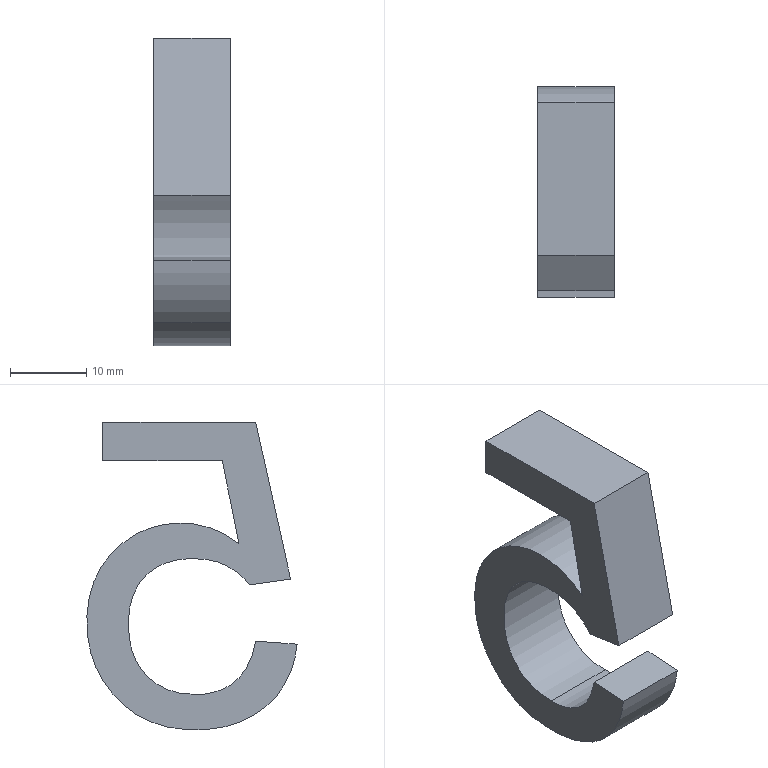Part | NX | features solid 2 | 1 solid | 14 faces | box 10 x 27.61 x 40.382 mm | volume 4846 mm3 | plane 9 | spline 5
STEP:
#1=CARTESIAN_POINT('',(2250.,-233.508,-587.73));
#2=VERTEX_POINT('',#1);
#3=CARTESIAN_POINT('',(2250.,-237.6,-579.522));
#4=VERTEX_POINT('',#3);
#5=CARTESIAN_POINT('',(2250.,-233.508,-587.73));
#6=CARTESIAN_POINT('',(2250.,-235.902,-585.686));
#7=CARTESIAN_POINT('',(2250.,-237.263,-582.948));
#8=CARTESIAN_POINT('',(2250.,-237.6,-579.522));
#9=B_SPLINE_CURVE_WITH_KNOTS('',3,(#5,#6,#7,#8),.UNSPECIFIED.,.F.,.F.,(4,4),(0.,0.04563),.PIECEWISE_BEZIER_KNOTS.);
#10=EDGE_CURVE('',#2,#4,#9,.T.);
#11=ORIENTED_EDGE('',*,*,#10,.F.);
#12=CARTESIAN_POINT('',(2260.,-233.508,-587.73));
#13=VERTEX_POINT('',#12);
#14=CARTESIAN_POINT('',(2260.,-233.508,-587.73));
#15=DIRECTION('',(-1.,0.,0.));
#16=VECTOR('',#15,1000.);
#17=LINE('',#14,#16);
#18=EDGE_CURVE('',#13,#2,#17,.T.);
#19=ORIENTED_EDGE('',*,*,#18,.F.);
#20=CARTESIAN_POINT('',(2260.,-237.6,-579.522));
#21=VERTEX_POINT('',#20);
#22=CARTESIAN_POINT('',(2260.,-233.508,-587.73));
#23=CARTESIAN_POINT('',(2260.,-235.902,-585.686));
#24=CARTESIAN_POINT('',(2260.,-237.263,-582.948));
#25=CARTESIAN_POINT('',(2260.,-237.6,-579.522));
#26=B_SPLINE_CURVE_WITH_KNOTS('',3,(#22,#23,#24,#25),.UNSPECIFIED.,.F.,.F.,(4,4),(0.,0.04563),.PIECEWISE_BEZIER_KNOTS.);
#27=EDGE_CURVE('',#13,#21,#26,.T.);
#28=ORIENTED_EDGE('',*,*,#27,.T.);
#29=CARTESIAN_POINT('',(2260.,-237.6,-579.522));
#30=DIRECTION('',(-1.,0.,0.));
#31=VECTOR('',#30,1000.);
#32=LINE('',#29,#31);
#33=EDGE_CURVE('',#21,#4,#32,.T.);
#34=ORIENTED_EDGE('',*,*,#33,.T.);
#35=EDGE_LOOP('',(#11,#19,#28,#34));
#36=FACE_BOUND('',#35,.T.);
#37=CARTESIAN_POINT('',(2260.,-233.508,-587.73));
#38=CARTESIAN_POINT('',(2250.,-233.508,-587.73));
#39=CARTESIAN_POINT('',(2260.,-235.902,-585.686));
#40=CARTESIAN_POINT('',(2250.,-235.902,-585.686));
#41=CARTESIAN_POINT('',(2260.,-237.263,-582.948));
#42=CARTESIAN_POINT('',(2250.,-237.263,-582.948));
#43=CARTESIAN_POINT('',(2260.,-237.6,-579.522));
#44=CARTESIAN_POINT('',(2250.,-237.6,-579.522));
#45=B_SPLINE_SURFACE_WITH_KNOTS('',3,1,((#37,#38),(#39,#40),(#41,#42),(#43,#44)),.SURF_OF_LINEAR_EXTRUSION.,.F.,.F.,.F.,(4,4),(2,2),(0.,0.04563),(0.,1.),.PIECEWISE_BEZIER_KNOTS.);
#46=ADVANCED_FACE('',(#36),#45,.T.);
#47=CARTESIAN_POINT('',(2250.,-232.17,-579.124));
#48=VERTEX_POINT('',#47);
#49=CARTESIAN_POINT('',(2250.,-237.6,-579.522));
#50=CARTESIAN_POINT('',(2250.,-235.79,-579.389));
#51=CARTESIAN_POINT('',(2250.,-233.98,-579.257));
#52=CARTESIAN_POINT('',(2250.,-232.17,-579.124));
#53=B_SPLINE_CURVE_WITH_KNOTS('',3,(#49,#50,#51,#52),.UNSPECIFIED.,.F.,.F.,(4,4),(0.04563,0.07202),.PIECEWISE_BEZIER_KNOTS.);
#54=EDGE_CURVE('',#4,#48,#53,.T.);
#55=ORIENTED_EDGE('',*,*,#54,.F.);
#56=ORIENTED_EDGE('',*,*,#33,.F.);
#57=CARTESIAN_POINT('',(2260.,-232.17,-579.124));
#58=VERTEX_POINT('',#57);
#59=CARTESIAN_POINT('',(2260.,-237.6,-579.522));
#60=CARTESIAN_POINT('',(2260.,-235.79,-579.389));
#61=CARTESIAN_POINT('',(2260.,-233.98,-579.257));
#62=CARTESIAN_POINT('',(2260.,-232.17,-579.124));
#63=B_SPLINE_CURVE_WITH_KNOTS('',3,(#59,#60,#61,#62),.UNSPECIFIED.,.F.,.F.,(4,4),(0.04563,0.07202),.PIECEWISE_BEZIER_KNOTS.);
#64=EDGE_CURVE('',#21,#58,#63,.T.);
#65=ORIENTED_EDGE('',*,*,#64,.T.);
#66=CARTESIAN_POINT('',(2260.,-232.17,-579.124));
#67=DIRECTION('',(-1.,0.,0.));
#68=VECTOR('',#67,1000.);
#69=LINE('',#66,#68);
#70=EDGE_CURVE('',#58,#48,#69,.T.);
#71=ORIENTED_EDGE('',*,*,#70,.T.);
#72=EDGE_LOOP('',(#55,#56,#65,#71));
#73=FACE_BOUND('',#72,.T.);
#74=CARTESIAN_POINT('',(2260.,-237.6,-579.522));
#75=DIRECTION('',(0.,-0.07304,0.9973));
#76=DIRECTION('',(0.,-0.9973,-0.07304));
#77=AXIS2_PLACEMENT_3D('',#74,#75,#76);
#78=PLANE('',#77);
#79=ADVANCED_FACE('',(#73),#78,.T.);
#80=CARTESIAN_POINT('',(2250.,-224.216,-586.115));
#81=VERTEX_POINT('',#80);
#82=CARTESIAN_POINT('',(2250.,-232.17,-579.124));
#83=CARTESIAN_POINT('',(2250.,-231.772,-581.48));
#84=CARTESIAN_POINT('',(2250.,-230.885,-583.239));
#85=CARTESIAN_POINT('',(2250.,-228.153,-585.572));
#86=CARTESIAN_POINT('',(2250.,-226.357,-586.145));
#87=CARTESIAN_POINT('',(2250.,-224.216,-586.115));
#88=B_SPLINE_CURVE_WITH_KNOTS('',3,(#82,#83,#84,#85,#86,#87),.UNSPECIFIED.,.F.,.F.,(4,2,4),(0.07202,0.1012,0.1307),.UNSPECIFIED.);
#89=EDGE_CURVE('',#48,#81,#88,.T.);
#90=ORIENTED_EDGE('',*,*,#89,.F.);
#91=ORIENTED_EDGE('',*,*,#70,.F.);
#92=CARTESIAN_POINT('',(2260.,-224.216,-586.115));
#93=VERTEX_POINT('',#92);
#94=CARTESIAN_POINT('',(2260.,-232.17,-579.124));
#95=CARTESIAN_POINT('',(2260.,-231.772,-581.48));
#96=CARTESIAN_POINT('',(2260.,-230.885,-583.239));
#97=CARTESIAN_POINT('',(2260.,-228.153,-585.572));
#98=CARTESIAN_POINT('',(2260.,-226.357,-586.145));
#99=CARTESIAN_POINT('',(2260.,-224.216,-586.115));
#100=B_SPLINE_CURVE_WITH_KNOTS('',3,(#94,#95,#96,#97,#98,#99),.UNSPECIFIED.,.F.,.F.,(4,2,4),(0.07202,0.1012,0.1307),.UNSPECIFIED.);
#101=EDGE_CURVE('',#58,#93,#100,.T.);
#102=ORIENTED_EDGE('',*,*,#101,.T.);
#103=CARTESIAN_POINT('',(2260.,-224.216,-586.115));
#104=DIRECTION('',(-1.,0.,0.));
#105=VECTOR('',#104,1000.);
#106=LINE('',#103,#105);
#107=EDGE_CURVE('',#93,#81,#106,.T.);
#108=ORIENTED_EDGE('',*,*,#107,.T.);
#109=EDGE_LOOP('',(#90,#91,#102,#108));
#110=FACE_BOUND('',#109,.T.);
#111=CARTESIAN_POINT('',(2260.,-232.17,-579.124));
#112=CARTESIAN_POINT('',(2250.,-232.17,-579.124));
#113=CARTESIAN_POINT('',(2260.,-231.372,-583.851));
#114=CARTESIAN_POINT('',(2250.,-231.372,-583.851));
#115=CARTESIAN_POINT('',(2260.,-228.485,-586.176));
#116=CARTESIAN_POINT('',(2250.,-228.485,-586.176));
#117=CARTESIAN_POINT('',(2260.,-224.216,-586.115));
#118=CARTESIAN_POINT('',(2250.,-224.216,-586.115));
#119=B_SPLINE_SURFACE_WITH_KNOTS('',3,1,((#111,#112),(#113,#114),(#115,#116),(#117,#118)),.SURF_OF_LINEAR_EXTRUSION.,.F.,.F.,.F.,(4,4),(2,2),(0.07202,0.1307),(0.,1.),.PIECEWISE_BEZIER_KNOTS.);
#120=ADVANCED_FACE('',(#110),#119,.T.);
#121=CARTESIAN_POINT('',(2250.,-231.328,-571.751));
#122=VERTEX_POINT('',#121);
#123=CARTESIAN_POINT('',(2250.,-224.216,-586.115));
#124=CARTESIAN_POINT('',(2250.,-221.554,-586.145));
#125=CARTESIAN_POINT('',(2250.,-219.413,-585.304));
#126=CARTESIAN_POINT('',(2250.,-217.799,-583.598));
#127=CARTESIAN_POINT('',(2250.,-216.216,-581.924));
#128=CARTESIAN_POINT('',(2250.,-215.436,-579.69));
#129=CARTESIAN_POINT('',(2250.,-215.436,-574.229));
#130=CARTESIAN_POINT('',(2250.,-216.17,-572.134));
#131=CARTESIAN_POINT('',(2250.,-219.122,-569.06));
#132=CARTESIAN_POINT('',(2250.,-221.233,-568.279));
#133=CARTESIAN_POINT('',(2250.,-224.002,-568.279));
#134=CARTESIAN_POINT('',(2250.,-225.73,-568.279));
#135=CARTESIAN_POINT('',(2250.,-227.229,-568.616));
#136=CARTESIAN_POINT('',(2250.,-229.627,-569.907));
#137=CARTESIAN_POINT('',(2250.,-230.594,-570.727));
#138=CARTESIAN_POINT('',(2250.,-231.328,-571.751));
#139=B_SPLINE_CURVE_WITH_KNOTS('',3,(#123,#124,#125,#126,#127,#128,#129,#130,#131,#132,#133,#134,#135,#136,#137,#138),.UNSPECIFIED.,.F.,.F.,(4,3,2,2,3,2,4),(0.1307,0.1656,0.2015,0.2352,0.2686,0.2911,0.3137),.UNSPECIFIED.);
#140=EDGE_CURVE('',#81,#122,#139,.T.);
#141=ORIENTED_EDGE('',*,*,#140,.F.);
#142=ORIENTED_EDGE('',*,*,#107,.F.);
#143=CARTESIAN_POINT('',(2260.,-231.328,-571.751));
#144=VERTEX_POINT('',#143);
#145=CARTESIAN_POINT('',(2260.,-224.216,-586.115));
#146=CARTESIAN_POINT('',(2260.,-221.554,-586.145));
#147=CARTESIAN_POINT('',(2260.,-219.413,-585.304));
#148=CARTESIAN_POINT('',(2260.,-217.799,-583.598));
#149=CARTESIAN_POINT('',(2260.,-216.216,-581.924));
#150=CARTESIAN_POINT('',(2260.,-215.436,-579.69));
#151=CARTESIAN_POINT('',(2260.,-215.436,-574.229));
#152=CARTESIAN_POINT('',(2260.,-216.17,-572.134));
#153=CARTESIAN_POINT('',(2260.,-219.122,-569.06));
#154=CARTESIAN_POINT('',(2260.,-221.233,-568.279));
#155=CARTESIAN_POINT('',(2260.,-224.002,-568.279));
#156=CARTESIAN_POINT('',(2260.,-225.73,-568.279));
#157=CARTESIAN_POINT('',(2260.,-227.229,-568.616));
#158=CARTESIAN_POINT('',(2260.,-229.627,-569.907));
#159=CARTESIAN_POINT('',(2260.,-230.594,-570.727));
#160=CARTESIAN_POINT('',(2260.,-231.328,-571.751));
#161=B_SPLINE_CURVE_WITH_KNOTS('',3,(#145,#146,#147,#148,#149,#150,#151,#152,#153,#154,#155,#156,#157,#158,#159,#160),.UNSPECIFIED.,.F.,.F.,(4,3,2,2,3,2,4),(0.1307,0.1656,0.2015,0.2352,0.2686,0.2911,0.3137),.UNSPECIFIED.);
#162=EDGE_CURVE('',#93,#144,#161,.T.);
#163=ORIENTED_EDGE('',*,*,#162,.T.);
#164=CARTESIAN_POINT('',(2260.,-231.328,-571.751));
#165=DIRECTION('',(-1.,0.,0.));
#166=VECTOR('',#165,1000.);
#167=LINE('',#164,#166);
#168=EDGE_CURVE('',#144,#122,#167,.T.);
#169=ORIENTED_EDGE('',*,*,#168,.T.);
#170=EDGE_LOOP('',(#141,#142,#163,#169));
#171=FACE_BOUND('',#170,.T.);
#172=CARTESIAN_POINT('',(2260.,-224.216,-586.115));
#173=CARTESIAN_POINT('',(2250.,-224.216,-586.115));
#174=CARTESIAN_POINT('',(2260.,-222.471,-586.135));
#175=CARTESIAN_POINT('',(2250.,-222.471,-586.135));
#176=CARTESIAN_POINT('',(2260.,-220.207,-585.624));
#177=CARTESIAN_POINT('',(2250.,-220.207,-585.624));
#178=CARTESIAN_POINT('',(2260.,-217.794,-583.741));
#179=CARTESIAN_POINT('',(2250.,-217.794,-583.741));
#180=CARTESIAN_POINT('',(2260.,-216.501,-581.979));
#181=CARTESIAN_POINT('',(2250.,-216.501,-581.979));
#182=CARTESIAN_POINT('',(2260.,-215.693,-579.891));
#183=CARTESIAN_POINT('',(2250.,-215.693,-579.891));
#184=CARTESIAN_POINT('',(2260.,-215.364,-577.41));
#185=CARTESIAN_POINT('',(2250.,-215.364,-577.41));
#186=CARTESIAN_POINT('',(2260.,-215.517,-574.731));
#187=CARTESIAN_POINT('',(2250.,-215.517,-574.731));
#188=CARTESIAN_POINT('',(2260.,-216.183,-572.568));
#189=CARTESIAN_POINT('',(2250.,-216.183,-572.568));
#190=CARTESIAN_POINT('',(2260.,-217.367,-570.739));
#191=CARTESIAN_POINT('',(2250.,-217.367,-570.739));
#192=CARTESIAN_POINT('',(2260.,-219.045,-569.339));
#193=CARTESIAN_POINT('',(2250.,-219.045,-569.339));
#194=CARTESIAN_POINT('',(2260.,-220.823,-568.637));
#195=CARTESIAN_POINT('',(2250.,-220.823,-568.637));
#196=CARTESIAN_POINT('',(2260.,-222.455,-568.342));
#197=CARTESIAN_POINT('',(2250.,-222.455,-568.342));
#198=CARTESIAN_POINT('',(2260.,-224.316,-568.23));
#199=CARTESIAN_POINT('',(2250.,-224.316,-568.23));
#200=CARTESIAN_POINT('',(2260.,-226.396,-568.42));
#201=CARTESIAN_POINT('',(2250.,-226.396,-568.42));
#202=CARTESIAN_POINT('',(2260.,-228.457,-569.176));
#203=CARTESIAN_POINT('',(2250.,-228.457,-569.176));
#204=CARTESIAN_POINT('',(2260.,-230.095,-570.309));
#205=CARTESIAN_POINT('',(2250.,-230.095,-570.309));
#206=CARTESIAN_POINT('',(2260.,-230.958,-571.234));
#207=CARTESIAN_POINT('',(2250.,-230.958,-571.234));
#208=CARTESIAN_POINT('',(2260.,-231.328,-571.751));
#209=CARTESIAN_POINT('',(2250.,-231.328,-571.751));
#210=B_SPLINE_SURFACE_WITH_KNOTS('',3,1,((#172,#173),(#174,#175),(#176,#177),(#178,#179),(#180,#181),(#182,#183),(#184,#185),(#186,#187),(#188,#189),(#190,#191),(#192,#193),(#194,#195),(#196,#197),(#198,#199),(#200,#201),(#202,#203),(#204,#205),(#206,#207),(#208,#209)),.SURF_OF_LINEAR_EXTRUSION.,.F.,.F.,.F.,(4,1,1,1,1,1,1,1,1,1,1,1,1,1,1,1,4),(2,2),(0.1307,0.1535,0.165,0.1764,0.1879,0.1993,0.2107,0.2222,0.2336,0.2451,0.2565,0.2622,0.268,0.2794,0.2908,0.3023,0.3137),(0.,1.),.UNSPECIFIED.);
#211=ADVANCED_FACE('',(#171),#210,.T.);
#212=CARTESIAN_POINT('',(2250.,-236.759,-570.971));
#213=VERTEX_POINT('',#212);
#214=CARTESIAN_POINT('',(2250.,-231.328,-571.751));
#215=CARTESIAN_POINT('',(2250.,-233.139,-571.491));
#216=CARTESIAN_POINT('',(2250.,-234.949,-571.231));
#217=CARTESIAN_POINT('',(2250.,-236.759,-570.971));
#218=B_SPLINE_CURVE_WITH_KNOTS('',3,(#214,#215,#216,#217),.UNSPECIFIED.,.F.,.F.,(4,4),(0.3137,0.341),.PIECEWISE_BEZIER_KNOTS.);
#219=EDGE_CURVE('',#122,#213,#218,.T.);
#220=ORIENTED_EDGE('',*,*,#219,.F.);
#221=ORIENTED_EDGE('',*,*,#168,.F.);
#222=CARTESIAN_POINT('',(2260.,-236.759,-570.971));
#223=VERTEX_POINT('',#222);
#224=CARTESIAN_POINT('',(2260.,-231.328,-571.751));
#225=CARTESIAN_POINT('',(2260.,-233.139,-571.491));
#226=CARTESIAN_POINT('',(2260.,-234.949,-571.231));
#227=CARTESIAN_POINT('',(2260.,-236.759,-570.971));
#228=B_SPLINE_CURVE_WITH_KNOTS('',3,(#224,#225,#226,#227),.UNSPECIFIED.,.F.,.F.,(4,4),(0.3137,0.341),.PIECEWISE_BEZIER_KNOTS.);
#229=EDGE_CURVE('',#144,#223,#228,.T.);
#230=ORIENTED_EDGE('',*,*,#229,.T.);
#231=CARTESIAN_POINT('',(2260.,-236.759,-570.971));
#232=DIRECTION('',(-1.,0.,0.));
#233=VECTOR('',#232,1000.);
#234=LINE('',#231,#233);
#235=EDGE_CURVE('',#223,#213,#234,.T.);
#236=ORIENTED_EDGE('',*,*,#235,.T.);
#237=EDGE_LOOP('',(#220,#221,#230,#236));
#238=FACE_BOUND('',#237,.T.);
#239=CARTESIAN_POINT('',(2260.,-231.328,-571.751));
#240=DIRECTION('',(0.,-0.1422,-0.9898));
#241=DIRECTION('',(0.,0.9898,-0.1422));
#242=AXIS2_PLACEMENT_3D('',#239,#240,#241);
#243=PLANE('',#242);
#244=ADVANCED_FACE('',(#238),#243,.T.);
#245=CARTESIAN_POINT('',(2250.,-232.17,-550.398));
#246=VERTEX_POINT('',#245);
#247=CARTESIAN_POINT('',(2250.,-236.759,-570.971));
#248=CARTESIAN_POINT('',(2250.,-235.229,-564.113));
#249=CARTESIAN_POINT('',(2250.,-233.699,-557.256));
#250=CARTESIAN_POINT('',(2250.,-232.17,-550.398));
#251=B_SPLINE_CURVE_WITH_KNOTS('',3,(#247,#248,#249,#250),.UNSPECIFIED.,.F.,.F.,(4,4),(0.341,0.4456),.PIECEWISE_BEZIER_KNOTS.);
#252=EDGE_CURVE('',#213,#246,#251,.T.);
#253=ORIENTED_EDGE('',*,*,#252,.F.);
#254=ORIENTED_EDGE('',*,*,#235,.F.);
#255=CARTESIAN_POINT('',(2260.,-232.17,-550.398));
#256=VERTEX_POINT('',#255);
#257=CARTESIAN_POINT('',(2260.,-236.759,-570.971));
#258=CARTESIAN_POINT('',(2260.,-235.229,-564.113));
#259=CARTESIAN_POINT('',(2260.,-233.699,-557.256));
#260=CARTESIAN_POINT('',(2260.,-232.17,-550.398));
#261=B_SPLINE_CURVE_WITH_KNOTS('',3,(#257,#258,#259,#260),.UNSPECIFIED.,.F.,.F.,(4,4),(0.341,0.4456),.PIECEWISE_BEZIER_KNOTS.);
#262=EDGE_CURVE('',#223,#256,#261,.T.);
#263=ORIENTED_EDGE('',*,*,#262,.T.);
#264=CARTESIAN_POINT('',(2260.,-232.17,-550.398));
#265=DIRECTION('',(-1.,0.,0.));
#266=VECTOR('',#265,1000.);
#267=LINE('',#264,#266);
#268=EDGE_CURVE('',#256,#246,#267,.T.);
#269=ORIENTED_EDGE('',*,*,#268,.T.);
#270=EDGE_LOOP('',(#253,#254,#263,#269));
#271=FACE_BOUND('',#270,.T.);
#272=CARTESIAN_POINT('',(2260.,-236.759,-570.971));
#273=DIRECTION('',(0.,-0.976,0.2177));
#274=DIRECTION('',(0.,-0.2177,-0.976));
#275=AXIS2_PLACEMENT_3D('',#272,#273,#274);
#276=PLANE('',#275);
#277=ADVANCED_FACE('',(#271),#276,.T.);
#278=CARTESIAN_POINT('',(2250.,-212.086,-550.398));
#279=VERTEX_POINT('',#278);
#280=CARTESIAN_POINT('',(2250.,-232.17,-550.398));
#281=CARTESIAN_POINT('',(2250.,-225.475,-550.398));
#282=CARTESIAN_POINT('',(2250.,-218.78,-550.398));
#283=CARTESIAN_POINT('',(2250.,-212.086,-550.398));
#284=B_SPLINE_CURVE_WITH_KNOTS('',3,(#280,#281,#282,#283),.UNSPECIFIED.,.F.,.F.,(4,4),(0.4456,0.5452),.PIECEWISE_BEZIER_KNOTS.);
#285=EDGE_CURVE('',#246,#279,#284,.T.);
#286=ORIENTED_EDGE('',*,*,#285,.F.);
#287=ORIENTED_EDGE('',*,*,#268,.F.);
#288=CARTESIAN_POINT('',(2260.,-212.086,-550.398));
#289=VERTEX_POINT('',#288);
#290=CARTESIAN_POINT('',(2260.,-232.17,-550.398));
#291=CARTESIAN_POINT('',(2260.,-225.475,-550.398));
#292=CARTESIAN_POINT('',(2260.,-218.78,-550.398));
#293=CARTESIAN_POINT('',(2260.,-212.086,-550.398));
#294=B_SPLINE_CURVE_WITH_KNOTS('',3,(#290,#291,#292,#293),.UNSPECIFIED.,.F.,.F.,(4,4),(0.4456,0.5452),.PIECEWISE_BEZIER_KNOTS.);
#295=EDGE_CURVE('',#256,#289,#294,.T.);
#296=ORIENTED_EDGE('',*,*,#295,.T.);
#297=CARTESIAN_POINT('',(2260.,-212.086,-550.398));
#298=DIRECTION('',(-1.,0.,0.));
#299=VECTOR('',#298,1000.);
#300=LINE('',#297,#299);
#301=EDGE_CURVE('',#289,#279,#300,.T.);
#302=ORIENTED_EDGE('',*,*,#301,.T.);
#303=EDGE_LOOP('',(#286,#287,#296,#302));
#304=FACE_BOUND('',#303,.T.);
#305=CARTESIAN_POINT('',(2260.,-232.17,-550.398));
#306=DIRECTION('',(0.,0.,1.));
#307=DIRECTION('',(1.,0.,0.));
#308=AXIS2_PLACEMENT_3D('',#305,#306,#307);
#309=PLANE('',#308);
#310=ADVANCED_FACE('',(#304),#309,.T.);
#311=CARTESIAN_POINT('',(2250.,-212.086,-555.446));
#312=VERTEX_POINT('',#311);
#313=CARTESIAN_POINT('',(2250.,-212.086,-550.398));
#314=CARTESIAN_POINT('',(2250.,-212.086,-552.08));
#315=CARTESIAN_POINT('',(2250.,-212.086,-553.763));
#316=CARTESIAN_POINT('',(2250.,-212.086,-555.446));
#317=B_SPLINE_CURVE_WITH_KNOTS('',3,(#313,#314,#315,#316),.UNSPECIFIED.,.F.,.F.,(4,4),(0.5452,0.5703),.PIECEWISE_BEZIER_KNOTS.);
#318=EDGE_CURVE('',#279,#312,#317,.T.);
#319=ORIENTED_EDGE('',*,*,#318,.F.);
#320=ORIENTED_EDGE('',*,*,#301,.F.);
#321=CARTESIAN_POINT('',(2260.,-212.086,-555.446));
#322=VERTEX_POINT('',#321);
#323=CARTESIAN_POINT('',(2260.,-212.086,-550.398));
#324=CARTESIAN_POINT('',(2260.,-212.086,-552.08));
#325=CARTESIAN_POINT('',(2260.,-212.086,-553.763));
#326=CARTESIAN_POINT('',(2260.,-212.086,-555.446));
#327=B_SPLINE_CURVE_WITH_KNOTS('',3,(#323,#324,#325,#326),.UNSPECIFIED.,.F.,.F.,(4,4),(0.5452,0.5703),.PIECEWISE_BEZIER_KNOTS.);
#328=EDGE_CURVE('',#289,#322,#327,.T.);
#329=ORIENTED_EDGE('',*,*,#328,.T.);
#330=CARTESIAN_POINT('',(2260.,-212.086,-555.446));
#331=DIRECTION('',(-1.,0.,0.));
#332=VECTOR('',#331,1000.);
#333=LINE('',#330,#332);
#334=EDGE_CURVE('',#322,#312,#333,.T.);
#335=ORIENTED_EDGE('',*,*,#334,.T.);
#336=EDGE_LOOP('',(#319,#320,#329,#335));
#337=FACE_BOUND('',#336,.T.);
#338=CARTESIAN_POINT('',(2260.,-212.086,-550.398));
#339=DIRECTION('',(0.,1.,0.));
#340=DIRECTION('',(-1.,0.,0.));
#341=AXIS2_PLACEMENT_3D('',#338,#339,#340);
#342=PLANE('',#341);
#343=ADVANCED_FACE('',(#337),#342,.T.);
#344=CARTESIAN_POINT('',(2250.,-227.78,-555.446));
#345=VERTEX_POINT('',#344);
#346=CARTESIAN_POINT('',(2250.,-212.086,-555.446));
#347=CARTESIAN_POINT('',(2250.,-217.317,-555.446));
#348=CARTESIAN_POINT('',(2250.,-222.548,-555.446));
#349=CARTESIAN_POINT('',(2250.,-227.78,-555.446));
#350=B_SPLINE_CURVE_WITH_KNOTS('',3,(#346,#347,#348,#349),.UNSPECIFIED.,.F.,.F.,(4,4),(0.5703,0.6481),.PIECEWISE_BEZIER_KNOTS.);
#351=EDGE_CURVE('',#312,#345,#350,.T.);
#352=ORIENTED_EDGE('',*,*,#351,.F.);
#353=ORIENTED_EDGE('',*,*,#334,.F.);
#354=CARTESIAN_POINT('',(2260.,-227.78,-555.446));
#355=VERTEX_POINT('',#354);
#356=CARTESIAN_POINT('',(2260.,-212.086,-555.446));
#357=CARTESIAN_POINT('',(2260.,-217.317,-555.446));
#358=CARTESIAN_POINT('',(2260.,-222.548,-555.446));
#359=CARTESIAN_POINT('',(2260.,-227.78,-555.446));
#360=B_SPLINE_CURVE_WITH_KNOTS('',3,(#356,#357,#358,#359),.UNSPECIFIED.,.F.,.F.,(4,4),(0.5703,0.6481),.PIECEWISE_BEZIER_KNOTS.);
#361=EDGE_CURVE('',#322,#355,#360,.T.);
#362=ORIENTED_EDGE('',*,*,#361,.T.);
#363=CARTESIAN_POINT('',(2260.,-227.78,-555.446));
#364=DIRECTION('',(-1.,0.,0.));
#365=VECTOR('',#364,1000.);
#366=LINE('',#363,#365);
#367=EDGE_CURVE('',#355,#345,#366,.T.);
#368=ORIENTED_EDGE('',*,*,#367,.T.);
#369=EDGE_LOOP('',(#352,#353,#362,#368));
#370=FACE_BOUND('',#369,.T.);
#371=CARTESIAN_POINT('',(2260.,-212.086,-555.446));
#372=DIRECTION('',(0.,0.,-1.));
#373=DIRECTION('',(-1.,0.,0.));
#374=AXIS2_PLACEMENT_3D('',#371,#372,#373);
#375=PLANE('',#374);
#376=ADVANCED_FACE('',(#370),#375,.T.);
#377=CARTESIAN_POINT('',(2250.,-229.967,-566.291));
#378=VERTEX_POINT('',#377);
#379=CARTESIAN_POINT('',(2250.,-227.78,-555.446));
#380=CARTESIAN_POINT('',(2250.,-228.509,-559.061));
#381=CARTESIAN_POINT('',(2250.,-229.238,-562.676));
#382=CARTESIAN_POINT('',(2250.,-229.967,-566.291));
#383=B_SPLINE_CURVE_WITH_KNOTS('',3,(#379,#380,#381,#382),.UNSPECIFIED.,.F.,.F.,(4,4),(0.6481,0.703),.PIECEWISE_BEZIER_KNOTS.);
#384=EDGE_CURVE('',#345,#378,#383,.T.);
#385=ORIENTED_EDGE('',*,*,#384,.F.);
#386=ORIENTED_EDGE('',*,*,#367,.F.);
#387=CARTESIAN_POINT('',(2260.,-229.967,-566.291));
#388=VERTEX_POINT('',#387);
#389=CARTESIAN_POINT('',(2260.,-227.78,-555.446));
#390=CARTESIAN_POINT('',(2260.,-228.509,-559.061));
#391=CARTESIAN_POINT('',(2260.,-229.238,-562.676));
#392=CARTESIAN_POINT('',(2260.,-229.967,-566.291));
#393=B_SPLINE_CURVE_WITH_KNOTS('',3,(#389,#390,#391,#392),.UNSPECIFIED.,.F.,.F.,(4,4),(0.6481,0.703),.PIECEWISE_BEZIER_KNOTS.);
#394=EDGE_CURVE('',#355,#388,#393,.T.);
#395=ORIENTED_EDGE('',*,*,#394,.T.);
#396=CARTESIAN_POINT('',(2260.,-229.967,-566.291));
#397=DIRECTION('',(-1.,0.,0.));
#398=VECTOR('',#397,1000.);
#399=LINE('',#396,#398);
#400=EDGE_CURVE('',#388,#378,#399,.T.);
#401=ORIENTED_EDGE('',*,*,#400,.T.);
#402=EDGE_LOOP('',(#385,#386,#395,#401));
#403=FACE_BOUND('',#402,.T.);
#404=CARTESIAN_POINT('',(2260.,-227.78,-555.446));
#405=DIRECTION('',(0.,0.9803,-0.1977));
#406=DIRECTION('',(0.,0.1977,0.9803));
#407=AXIS2_PLACEMENT_3D('',#404,#405,#406);
#408=PLANE('',#407);
#409=ADVANCED_FACE('',(#403),#408,.T.);
#410=CARTESIAN_POINT('',(2250.,-213.294,-585.931));
#411=VERTEX_POINT('',#410);
#412=CARTESIAN_POINT('',(2250.,-229.967,-566.291));
#413=CARTESIAN_POINT('',(2250.,-227.566,-564.516));
#414=CARTESIAN_POINT('',(2250.,-225.057,-563.614));
#415=CARTESIAN_POINT('',(2250.,-222.441,-563.614));
#416=CARTESIAN_POINT('',(2250.,-218.938,-563.614));
#417=CARTESIAN_POINT('',(2250.,-215.986,-564.837));
#418=CARTESIAN_POINT('',(2250.,-211.16,-569.663));
#419=CARTESIAN_POINT('',(2250.,-209.99,-572.776));
#420=CARTESIAN_POINT('',(2250.,-209.99,-580.195));
#421=CARTESIAN_POINT('',(2250.,-211.091,-583.331));
#422=CARTESIAN_POINT('',(2250.,-213.294,-585.931));
#423=B_SPLINE_CURVE_WITH_KNOTS('',3,(#412,#413,#414,#415,#416,#417,#418,#419,#420,#421,#422),.UNSPECIFIED.,.F.,.F.,(4,3,2,2,4),(0.703,0.7434,0.7922,0.8415,0.889),.UNSPECIFIED.);
#424=EDGE_CURVE('',#378,#411,#423,.T.);
#425=ORIENTED_EDGE('',*,*,#424,.F.);
#426=ORIENTED_EDGE('',*,*,#400,.F.);
#427=CARTESIAN_POINT('',(2260.,-213.294,-585.931));
#428=VERTEX_POINT('',#427);
#429=CARTESIAN_POINT('',(2260.,-229.967,-566.291));
#430=CARTESIAN_POINT('',(2260.,-227.566,-564.516));
#431=CARTESIAN_POINT('',(2260.,-225.057,-563.614));
#432=CARTESIAN_POINT('',(2260.,-222.441,-563.614));
#433=CARTESIAN_POINT('',(2260.,-218.938,-563.614));
#434=CARTESIAN_POINT('',(2260.,-215.986,-564.837));
#435=CARTESIAN_POINT('',(2260.,-211.16,-569.663));
#436=CARTESIAN_POINT('',(2260.,-209.99,-572.776));
#437=CARTESIAN_POINT('',(2260.,-209.99,-580.195));
#438=CARTESIAN_POINT('',(2260.,-211.091,-583.331));
#439=CARTESIAN_POINT('',(2260.,-213.294,-585.931));
#440=B_SPLINE_CURVE_WITH_KNOTS('',3,(#429,#430,#431,#432,#433,#434,#435,#436,#437,#438,#439),.UNSPECIFIED.,.F.,.F.,(4,3,2,2,4),(0.703,0.7434,0.7922,0.8415,0.889),.UNSPECIFIED.);
#441=EDGE_CURVE('',#388,#428,#440,.T.);
#442=ORIENTED_EDGE('',*,*,#441,.T.);
#443=CARTESIAN_POINT('',(2260.,-213.294,-585.931));
#444=DIRECTION('',(-1.,0.,0.));
#445=VECTOR('',#444,1000.);
#446=LINE('',#443,#445);
#447=EDGE_CURVE('',#428,#411,#446,.T.);
#448=ORIENTED_EDGE('',*,*,#447,.T.);
#449=EDGE_LOOP('',(#425,#426,#442,#448));
#450=FACE_BOUND('',#449,.T.);
#451=CARTESIAN_POINT('',(2260.,-229.967,-566.291));
#452=CARTESIAN_POINT('',(2250.,-229.967,-566.291));
#453=CARTESIAN_POINT('',(2260.,-228.584,-565.268));
#454=CARTESIAN_POINT('',(2250.,-228.584,-565.268));
#455=CARTESIAN_POINT('',(2260.,-226.463,-564.17));
#456=CARTESIAN_POINT('',(2250.,-226.463,-564.17));
#457=CARTESIAN_POINT('',(2260.,-223.868,-563.661));
#458=CARTESIAN_POINT('',(2250.,-223.868,-563.661));
#459=CARTESIAN_POINT('',(2260.,-222.398,-563.596));
#460=CARTESIAN_POINT('',(2250.,-222.398,-563.596));
#461=CARTESIAN_POINT('',(2260.,-220.709,-563.674));
#462=CARTESIAN_POINT('',(2250.,-220.709,-563.674));
#463=CARTESIAN_POINT('',(2260.,-218.813,-564.029));
#464=CARTESIAN_POINT('',(2250.,-218.813,-564.029));
#465=CARTESIAN_POINT('',(2260.,-216.68,-564.867));
#466=CARTESIAN_POINT('',(2250.,-216.68,-564.867));
#467=CARTESIAN_POINT('',(2260.,-214.756,-566.105));
#468=CARTESIAN_POINT('',(2250.,-214.756,-566.105));
#469=CARTESIAN_POINT('',(2260.,-212.384,-568.329));
#470=CARTESIAN_POINT('',(2250.,-212.384,-568.329));
#471=CARTESIAN_POINT('',(2260.,-210.83,-571.032));
#472=CARTESIAN_POINT('',(2250.,-210.83,-571.032));
#473=CARTESIAN_POINT('',(2260.,-210.088,-574.158));
#474=CARTESIAN_POINT('',(2250.,-210.088,-574.158));
#475=CARTESIAN_POINT('',(2260.,-209.926,-576.791));
#476=CARTESIAN_POINT('',(2250.,-209.926,-576.791));
#477=CARTESIAN_POINT('',(2260.,-210.158,-579.388));
#478=CARTESIAN_POINT('',(2250.,-210.158,-579.388));
#479=CARTESIAN_POINT('',(2260.,-210.995,-582.553));
#480=CARTESIAN_POINT('',(2250.,-210.995,-582.553));
#481=CARTESIAN_POINT('',(2260.,-212.216,-584.658));
#482=CARTESIAN_POINT('',(2250.,-212.216,-584.658));
#483=CARTESIAN_POINT('',(2260.,-213.294,-585.931));
#484=CARTESIAN_POINT('',(2250.,-213.294,-585.931));
#485=B_SPLINE_SURFACE_WITH_KNOTS('',3,1,((#451,#452),(#453,#454),(#455,#456),(#457,#458),(#459,#460),(#461,#462),(#463,#464),(#465,#466),(#467,#468),(#469,#470),(#471,#472),(#473,#474),(#475,#476),(#477,#478),(#479,#480),(#481,#482),(#483,#484)),.SURF_OF_LINEAR_EXTRUSION.,.F.,.F.,.F.,(4,1,1,1,1,1,1,1,1,1,1,1,1,1,4),(2,2),(0.703,0.7263,0.7379,0.7437,0.7495,0.7612,0.7728,0.7844,0.796,0.8193,0.8309,0.8425,0.8541,0.8658,0.889),(0.,1.),.UNSPECIFIED.);
#486=ADVANCED_FACE('',(#450),#485,.T.);
#487=CARTESIAN_POINT('',(2250.,-213.294,-585.931));
#488=CARTESIAN_POINT('',(2250.,-215.956,-589.174));
#489=CARTESIAN_POINT('',(2250.,-219.611,-590.78));
#490=CARTESIAN_POINT('',(2250.,-228.009,-590.78));
#491=CARTESIAN_POINT('',(2250.,-231.099,-589.786));
#492=CARTESIAN_POINT('',(2250.,-233.508,-587.73));
#493=B_SPLINE_CURVE_WITH_KNOTS('',3,(#487,#488,#489,#490,#491,#492),.UNSPECIFIED.,.F.,.F.,(4,2,4),(0.889,0.9503,1.),.UNSPECIFIED.);
#494=EDGE_CURVE('',#411,#2,#493,.T.);
#495=ORIENTED_EDGE('',*,*,#494,.F.);
#496=ORIENTED_EDGE('',*,*,#447,.F.);
#497=CARTESIAN_POINT('',(2260.,-213.294,-585.931));
#498=CARTESIAN_POINT('',(2260.,-215.956,-589.174));
#499=CARTESIAN_POINT('',(2260.,-219.611,-590.78));
#500=CARTESIAN_POINT('',(2260.,-228.009,-590.78));
#501=CARTESIAN_POINT('',(2260.,-231.099,-589.786));
#502=CARTESIAN_POINT('',(2260.,-233.508,-587.73));
#503=B_SPLINE_CURVE_WITH_KNOTS('',3,(#497,#498,#499,#500,#501,#502),.UNSPECIFIED.,.F.,.F.,(4,2,4),(0.889,0.9503,1.),.UNSPECIFIED.);
#504=EDGE_CURVE('',#428,#13,#503,.T.);
#505=ORIENTED_EDGE('',*,*,#504,.T.);
#506=ORIENTED_EDGE('',*,*,#18,.T.);
#507=EDGE_LOOP('',(#495,#496,#505,#506));
#508=FACE_BOUND('',#507,.T.);
#509=CARTESIAN_POINT('',(2260.,-213.294,-585.931));
#510=CARTESIAN_POINT('',(2250.,-213.294,-585.931));
#511=CARTESIAN_POINT('',(2260.,-214.5,-587.4));
#512=CARTESIAN_POINT('',(2250.,-214.5,-587.4));
#513=CARTESIAN_POINT('',(2260.,-217.321,-589.666));
#514=CARTESIAN_POINT('',(2250.,-217.321,-589.666));
#515=CARTESIAN_POINT('',(2260.,-221.85,-590.834));
#516=CARTESIAN_POINT('',(2250.,-221.85,-590.834));
#517=CARTESIAN_POINT('',(2260.,-226.1,-590.778));
#518=CARTESIAN_POINT('',(2250.,-226.1,-590.778));
#519=CARTESIAN_POINT('',(2260.,-229.822,-590.102));
#520=CARTESIAN_POINT('',(2250.,-229.822,-590.102));
#521=CARTESIAN_POINT('',(2260.,-232.164,-588.877));
#522=CARTESIAN_POINT('',(2250.,-232.164,-588.877));
#523=CARTESIAN_POINT('',(2260.,-233.508,-587.73));
#524=CARTESIAN_POINT('',(2250.,-233.508,-587.73));
#525=B_SPLINE_SURFACE_WITH_KNOTS('',3,1,((#509,#510),(#511,#512),(#513,#514),(#515,#516),(#517,#518),(#519,#520),(#521,#522),(#523,#524)),.SURF_OF_LINEAR_EXTRUSION.,.F.,.F.,.F.,(4,1,1,1,1,4),(2,2),(0.889,0.9168,0.9445,0.9584,0.9723,1.),(0.,1.),.UNSPECIFIED.);
#526=ADVANCED_FACE('',(#508),#525,.T.);
#527=ORIENTED_EDGE('',*,*,#27,.F.);
#528=ORIENTED_EDGE('',*,*,#504,.F.);
#529=ORIENTED_EDGE('',*,*,#441,.F.);
#530=ORIENTED_EDGE('',*,*,#394,.F.);
#531=ORIENTED_EDGE('',*,*,#361,.F.);
#532=ORIENTED_EDGE('',*,*,#328,.F.);
#533=ORIENTED_EDGE('',*,*,#295,.F.);
#534=ORIENTED_EDGE('',*,*,#262,.F.);
#535=ORIENTED_EDGE('',*,*,#229,.F.);
#536=ORIENTED_EDGE('',*,*,#162,.F.);
#537=ORIENTED_EDGE('',*,*,#101,.F.);
#538=ORIENTED_EDGE('',*,*,#64,.F.);
#539=EDGE_LOOP('',(#527,#528,#529,#530,#531,#532,#533,#534,#535,#536,#537,#538));
#540=FACE_BOUND('',#539,.T.);
#541=CARTESIAN_POINT('',(2260.,-236.326,-584.145));
#542=DIRECTION('',(1.,0.,0.));
#543=DIRECTION('',(0.,1.,0.));
#544=AXIS2_PLACEMENT_3D('',#541,#542,#543);
#545=PLANE('',#544);
#546=ADVANCED_FACE('',(#540),#545,.T.);
#547=ORIENTED_EDGE('',*,*,#10,.T.);
#548=ORIENTED_EDGE('',*,*,#54,.T.);
#549=ORIENTED_EDGE('',*,*,#89,.T.);
#550=ORIENTED_EDGE('',*,*,#140,.T.);
#551=ORIENTED_EDGE('',*,*,#219,.T.);
#552=ORIENTED_EDGE('',*,*,#252,.T.);
#553=ORIENTED_EDGE('',*,*,#285,.T.);
#554=ORIENTED_EDGE('',*,*,#318,.T.);
#555=ORIENTED_EDGE('',*,*,#351,.T.);
#556=ORIENTED_EDGE('',*,*,#384,.T.);
#557=ORIENTED_EDGE('',*,*,#424,.T.);
#558=ORIENTED_EDGE('',*,*,#494,.T.);
#559=EDGE_LOOP('',(#547,#548,#549,#550,#551,#552,#553,#554,#555,#556,#557,#558));
#560=FACE_BOUND('',#559,.T.);
#561=CARTESIAN_POINT('',(2250.,-236.326,-584.145));
#562=DIRECTION('',(1.,0.,0.));
#563=DIRECTION('',(0.,1.,0.));
#564=AXIS2_PLACEMENT_3D('',#561,#562,#563);
#565=PLANE('',#564);
#566=ADVANCED_FACE('',(#560),#565,.F.);
#567=CLOSED_SHELL('',(#46,#79,#120,#211,#244,#277,#310,#343,#376,#409,#486,#526,#546,#566));
#568=MANIFOLD_SOLID_BREP('',#567);
#569=(LENGTH_UNIT()NAMED_UNIT(*)SI_UNIT(.MILLI.,.METRE.));
#570=UNCERTAINTY_MEASURE_WITH_UNIT(LENGTH_MEASURE(0.0508),#569,'','');
#571=(NAMED_UNIT(*)PLANE_ANGLE_UNIT()SI_UNIT($,.RADIAN.));
#572=(NAMED_UNIT(*)SI_UNIT($,.STERADIAN.)SOLID_ANGLE_UNIT());
#573=(GEOMETRIC_REPRESENTATION_CONTEXT(3)GLOBAL_UNCERTAINTY_ASSIGNED_CONTEXT((#570))GLOBAL_UNIT_ASSIGNED_CONTEXT((#569,#571,#572))REPRESENTATION_CONTEXT('',''));
#574=ADVANCED_BREP_SHAPE_REPRESENTATION('',(#568),#573);